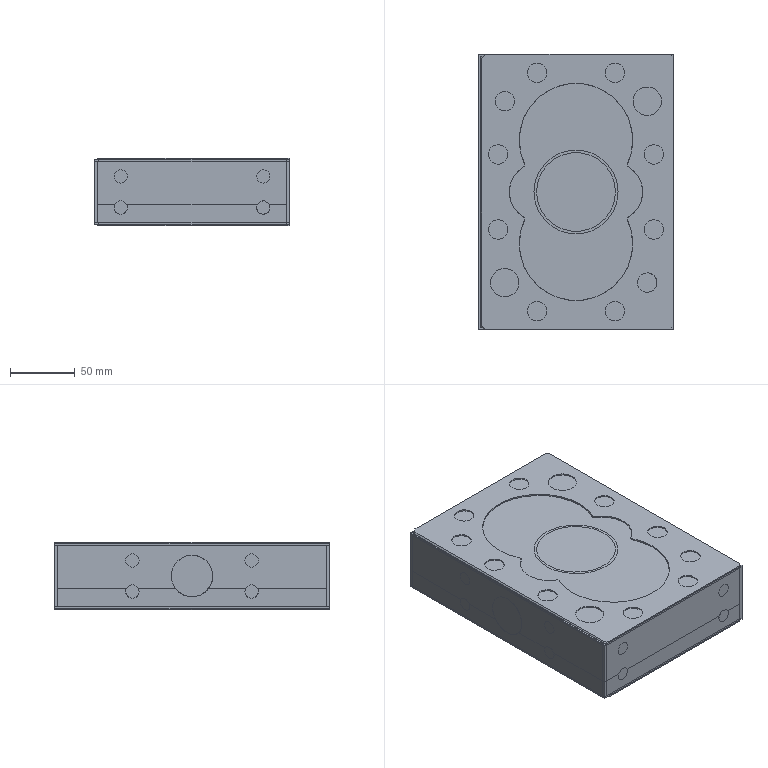CAM job | NX | 3-axis milling, drilling | part box 150.2 x 212.2 x 52.4 mm | stock box 150.2 x 212.2 x 52.4 mm
Tools:
number,name,description,diameter,corner_radius,flute_length,length,flutes
0,D17R0.8圆鼻飞刀,Milling Tool-5 Parameters,17.0,0.8,60.0,60.0,2
0,D6点孔钻,Drilling Tool,10.0,0.0,5.0,40.0,2
6,D45R0.8圆鼻飞刀,Milling Tool-5 Parameters,45.0,0.8,50.0,50.0,3
0,D6点孔钻_1,Drilling Tool,10.0,0.0,5.0,40.0,2
0,Z10.3钻头,Drilling Tool,20.0,0.0,35.0,50.0,2
2,Z8.5钻头,Drilling Tool,15.0,0.0,35.0,50.0,2
0,Z1.6钻头,Drilling Tool,10.2,0.0,35.0,50.0,2
0,Z3.3钻头,Drilling Tool,40.0,0.0,35.0,50.0,2
6,D10平底刀,Milling Tool-5 Parameters,10.0,0.0,22.0,25.0,4
0,Z8.5钻头_1,Drilling Tool,8.5,0.0,35.0,50.0,2
0,D8平底刀,Milling Tool-5 Parameters,8.0,0.0,20.0,23.0,4
0,D21R0.8圆鼻飞刀,Milling Tool-5 Parameters,25.0,0.8,50.0,50.0,2
0,D16平底刀,Milling Tool-5 Parameters,32.0,0.0,50.0,55.0,4
Operations:
program,operation,operation_type,tool,method,geometry_group,spindle_rpm,surface_speed,feed_per_tooth,feed_cut,feed_plunge,cut_length_mm,path_length_mm,cut_time_min,machine_time_min
图层30,G81点孔_5,Operation,D6点孔钻_1,METHOD,MCS,1500.0,47.0,0.02,60.0,0.0,3.0,46.0,0.05,0.0543
图层30,G83钻孔_3,Operation,Z8.5钻头_1,METHOD,MCS,800.0,21.0,0.0375,60.0,0.0,15.5,71.0,0.2583,0.2639
图层30,孔铣开粗_4,CylinderMilling,D8平底刀,METHOD,MCS,1500.0,37.0,0.0333,200.0,80.0,135.787,189.587,0.6807,0.6861
.NC,边界倒角,PlanarMilling,D6点孔钻,METHOD,WORKPIECE---A,2000.0,62.0,0.125,500.0,80.0,738.142,940.742,1.478,1.498
.NC,边界倒角_COPY,PlanarMilling,D6点孔钻,METHOD,WORKPIECE---A,2000.0,62.0,0.125,500.0,80.0,33.011,1347.054,0.0712,0.2026
.NC_1,G81点孔_6,Operation,Z3.3钻头,METHOD,WORKPIECE---A,300.0,37.0,0.0167,10.0,0.0,160.5,644.042,16.05,16.098
.NC_1,PLANAR_PROFILE,PlanarMilling,D45R0.8圆鼻飞刀,METHOD,WORKPIECE---A,1061.0,150.0,0.4,1273.2,100.0,30164.399,30414.199,23.692,23.717
.NC_1,G81点孔,Operation,D6点孔钻_1,METHOD,WORKPIECE---A,1500.0,47.0,0.02,60.0,0.0,36.0,2574.199,0.6,0.8538
.NC_1,G83钻孔,Operation,Z8.5钻头,METHOD,WORKPIECE---A,800.0,37.0,0.0187,30.0,0.0,535.0,3235.19,17.833,18.103
.NC_1,G81点孔_1,Operation,Z10.3钻头,METHOD,WORKPIECE---A,500.0,31.0,0.02,20.0,0.0,107.0,718.206,5.35,5.411
.NC_1,孔铣开粗,CylinderMilling,D17R0.8圆鼻飞刀,METHOD,WORKPIECE---A,1500.0,80.0,0.4,1200.0,80.0,5801.811,6447.456,4.837,4.902
.NC_1,孔铣开粗_1,CylinderMilling,D17R0.8圆鼻飞刀,METHOD,WORKPIECE---A,1500.0,80.0,0.2667,800.0,80.0,1913.639,2662.083,2.394,2.469
.NC_1,等高外形,ZLevelMilling,D17R0.8圆鼻飞刀,METHOD,WORKPIECE---A,2750.0,146.0,0.5,2750.0,80.0,42237.636,42488.834,15.36,15.385
5,G81点孔_2,Operation,D6点孔钻_1,METHOD,MCS---C,2500.0,235.0,0.024,120.0,0.0,15.0,219.22,0.125,0.1454
5,G81点孔_3,Operation,Z3.3钻头,METHOD,MCS---C,500.0,5.0,0.02,20.0,0.0,31.5,103.0,1.575,1.582
5,孔铣开粗_3,CylinderMilling,D21R0.8圆鼻飞刀,METHOD,MCS---C,2000.0,106.0,0.375,1500.0,80.0,3570.024,3643.824,2.381,2.388
5,G81点孔_7,Operation,D16平底刀,METHOD,MCS---C,500.0,50.0,0.025,50.0,0.0,33.281,106.561,0.6656,0.6729
5,G83钻孔_1,Operation,Z1.6钻头,METHOD,MCS---C,800.0,25.0,0.0262,42.0,0.0,86.0,498.694,2.048,2.089
5,孔铣开粗_2,CylinderMilling,D10平底刀,METHOD,MCS---C,1700.0,53.0,0.0294,200.0,80.0,456.702,911.903,2.29,2.335
6,G81点孔_4,Operation,D6点孔钻_1,METHOD,MCS---D,1500.0,47.0,0.02,60.0,0.0,12.0,312.567,0.2,0.2301
6,G83钻孔_2,Operation,Z1.6钻头,METHOD,MCS---D,800.0,25.0,0.0262,42.0,0.0,139.022,566.611,3.31,3.353